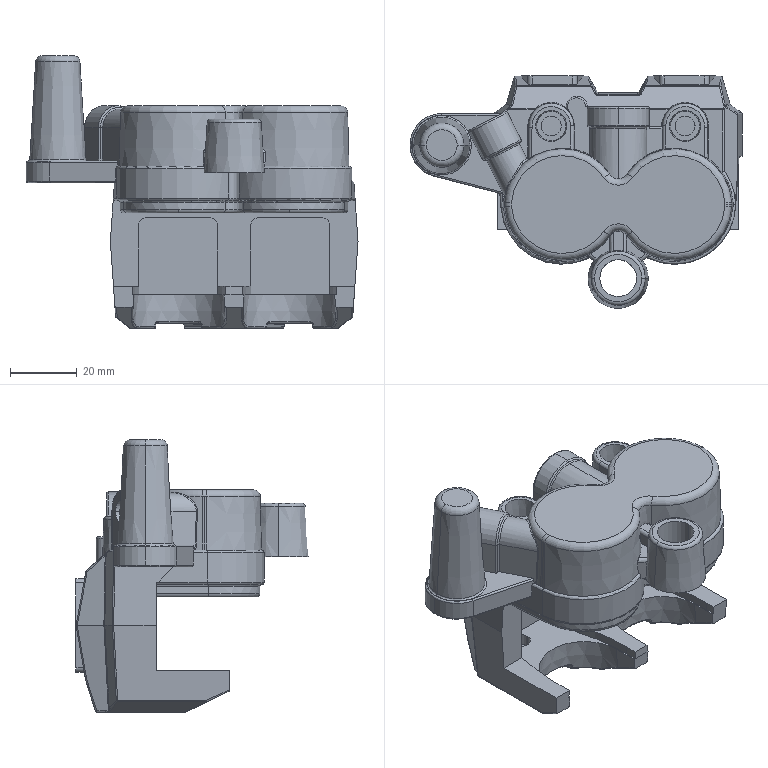Part | SolidWorks | features BaseBody 1 | 1 solid | 476 faces | box 99.2 x 69.5 x 81.512 mm | volume 106947 mm3 | cylinder 185 | plane 147 | torus 53 | spline 40 | sphere 28 | cone 23 | commonest cylinder face diameters 1 x108 2 x10 3 x8 6 x8 4 x6 1.5 x4